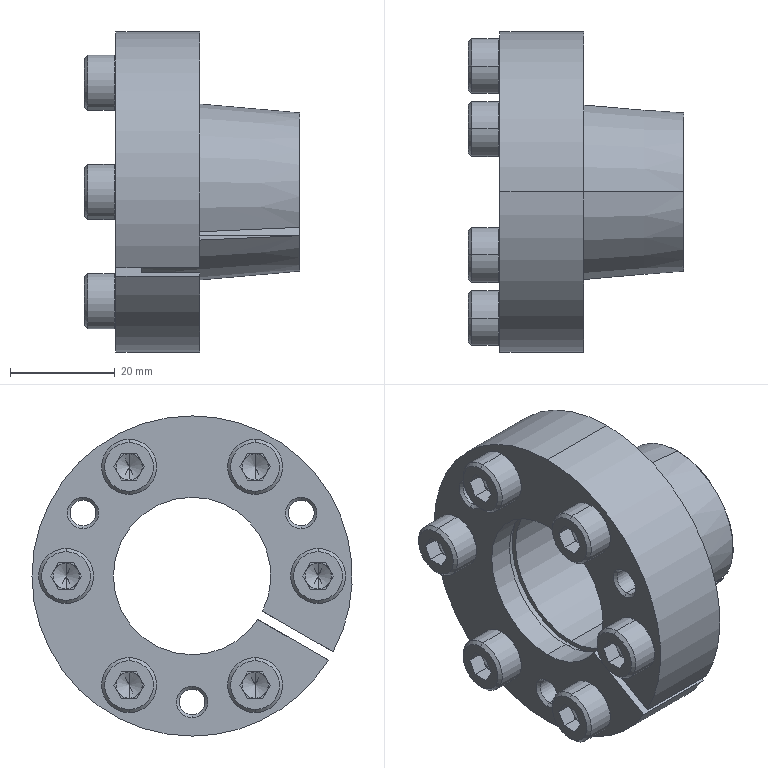Part | STEP file | MLR30bonnet | 1 solid | 200 faces | box 41 x 61 x 61 mm | volume 20958 mm3 | plane 92 | cone 63 | cylinder 45 | commonest cylinder face diameters 6 x12 10.5 x12 4.917 x6 30 x6 31.8 x3 58.56 x3